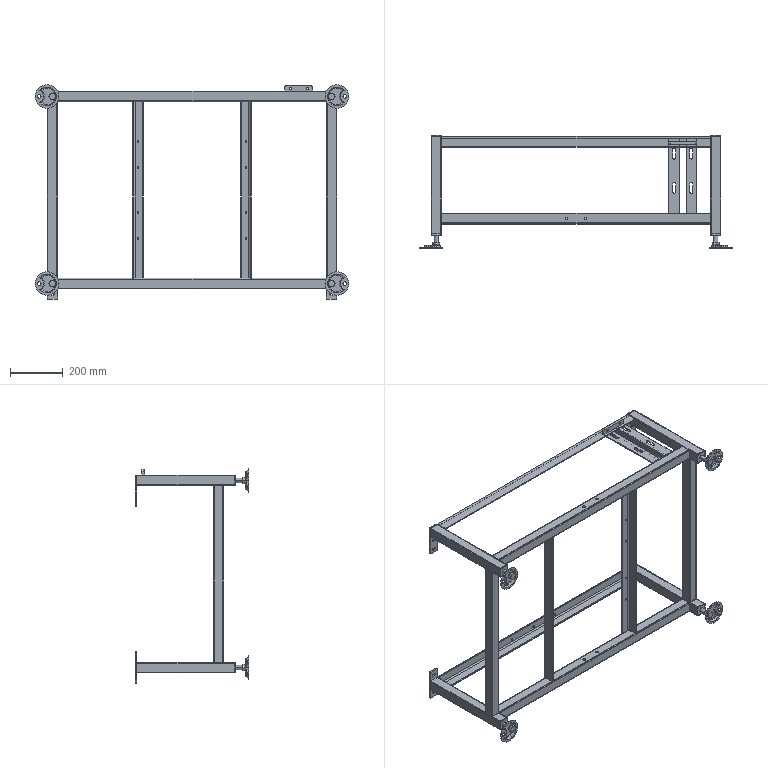Part | SolidWorks | 28 solids | 749 faces | box 1190 x 430 x 815 mm | volume 2877234 mm3 | plane 328 | cylinder 269 | cone 80 | sphere 32 | torus 24 | spline 16 | commonest cylinder face diameters 9 x50 6 x40 2 x26 10 x25 3 x24 6.8 x16